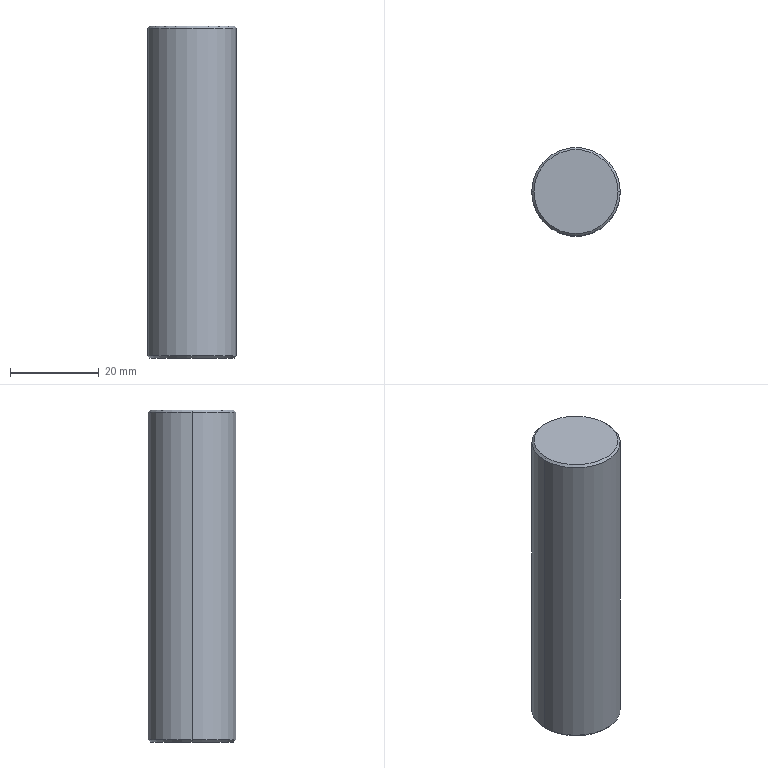Part | Creo | 1 solid | 15 faces | box 20 x 20 x 75 mm | volume 22497 mm3 | cone 6 | cylinder 6 | plane 3 | commonest cylinder face diameters 6.7 x2 8 x2 20 x2
STEP:
#1=CARTESIAN_POINT('',(259.5,184.,-188.491));
#2=VERTEX_POINT('',#1);
#3=CARTESIAN_POINT('',(240.5,184.,-188.491));
#4=VERTEX_POINT('',#3);
#5=CARTESIAN_POINT('',(250.,184.,-188.491));
#6=DIRECTION('',(0.,0.,-1.));
#7=DIRECTION('',(1.,0.,0.));
#8=AXIS2_PLACEMENT_3D('',#5,#6,#7);
#9=CIRCLE('',#8,9.5);
#10=EDGE_CURVE('',#2,#4,#9,.T.);
#11=ORIENTED_EDGE('',*,*,#10,.F.);
#12=CARTESIAN_POINT('',(250.,184.,-188.491));
#13=DIRECTION('',(0.,0.,-1.));
#14=DIRECTION('',(-1.,0.,0.));
#15=AXIS2_PLACEMENT_3D('',#12,#13,#14);
#16=CIRCLE('',#15,9.5);
#17=EDGE_CURVE('',#4,#2,#16,.T.);
#18=ORIENTED_EDGE('',*,*,#17,.F.);
#19=EDGE_LOOP('',(#11,#18));
#20=FACE_OUTER_BOUND('',#19,.F.);
#21=CARTESIAN_POINT('',(246.,184.,-188.491));
#22=VERTEX_POINT('',#21);
#23=CARTESIAN_POINT('',(254.,184.,-188.491));
#24=VERTEX_POINT('',#23);
#25=CARTESIAN_POINT('',(250.,184.,-188.491));
#26=DIRECTION('',(0.,0.,1.));
#27=DIRECTION('',(-1.,0.,0.));
#28=AXIS2_PLACEMENT_3D('',#25,#26,#27);
#29=CIRCLE('',#28,4.);
#30=EDGE_CURVE('',#22,#24,#29,.T.);
#31=ORIENTED_EDGE('',*,*,#30,.F.);
#32=CARTESIAN_POINT('',(250.,184.,-188.491));
#33=DIRECTION('',(0.,0.,1.));
#34=DIRECTION('',(1.,0.,0.));
#35=AXIS2_PLACEMENT_3D('',#32,#33,#34);
#36=CIRCLE('',#35,4.);
#37=EDGE_CURVE('',#24,#22,#36,.T.);
#38=ORIENTED_EDGE('',*,*,#37,.F.);
#39=EDGE_LOOP('',(#31,#38));
#40=FACE_BOUND('',#39,.F.);
#41=CARTESIAN_POINT('',(250.,184.,-188.491));
#42=DIRECTION('',(0.,0.,-1.));
#43=DIRECTION('',(-1.,0.,0.));
#44=AXIS2_PLACEMENT_3D('',#41,#42,#43);
#45=PLANE('',#44);
#46=ADVANCED_FACE('',(#20,#40),#45,.T.);
#47=ORIENTED_EDGE('',*,*,#10,.T.);
#48=CARTESIAN_POINT('',(240.,184.,-187.991));
#49=VERTEX_POINT('',#48);
#50=CARTESIAN_POINT('',(240.5,184.,-188.491));
#51=DIRECTION('',(-0.7071,0.,0.7071));
#52=VECTOR('',#51,0.7071);
#53=LINE('',#50,#52);
#54=EDGE_CURVE('',#4,#49,#53,.T.);
#55=ORIENTED_EDGE('',*,*,#54,.T.);
#56=CARTESIAN_POINT('',(260.,184.,-187.991));
#57=VERTEX_POINT('',#56);
#58=CARTESIAN_POINT('',(250.,184.,-187.991));
#59=DIRECTION('',(0.,0.,-1.));
#60=DIRECTION('',(1.,0.,0.));
#61=AXIS2_PLACEMENT_3D('',#58,#59,#60);
#62=CIRCLE('',#61,10.);
#63=EDGE_CURVE('',#57,#49,#62,.T.);
#64=ORIENTED_EDGE('',*,*,#63,.F.);
#65=CARTESIAN_POINT('',(259.5,184.,-188.491));
#66=DIRECTION('',(0.7071,0.,0.7071));
#67=VECTOR('',#66,0.7071);
#68=LINE('',#65,#67);
#69=EDGE_CURVE('',#2,#57,#68,.T.);
#70=ORIENTED_EDGE('',*,*,#69,.F.);
#71=EDGE_LOOP('',(#47,#55,#64,#70));
#72=FACE_OUTER_BOUND('',#71,.F.);
#73=CARTESIAN_POINT('',(250.,184.,-188.241));
#74=DIRECTION('',(0.,0.,1.));
#75=DIRECTION('',(1.,0.,0.));
#76=AXIS2_PLACEMENT_3D('',#73,#74,#75);
#77=CONICAL_SURFACE('',#76,9.75,45.);
#78=ADVANCED_FACE('',(#72),#77,.T.);
#79=ORIENTED_EDGE('',*,*,#17,.T.);
#80=ORIENTED_EDGE('',*,*,#69,.T.);
#81=CARTESIAN_POINT('',(250.,184.,-187.991));
#82=DIRECTION('',(0.,0.,-1.));
#83=DIRECTION('',(-1.,0.,0.));
#84=AXIS2_PLACEMENT_3D('',#81,#82,#83);
#85=CIRCLE('',#84,10.);
#86=EDGE_CURVE('',#49,#57,#85,.T.);
#87=ORIENTED_EDGE('',*,*,#86,.F.);
#88=ORIENTED_EDGE('',*,*,#54,.F.);
#89=EDGE_LOOP('',(#79,#80,#87,#88));
#90=FACE_OUTER_BOUND('',#89,.F.);
#91=CARTESIAN_POINT('',(250.,184.,-188.241));
#92=DIRECTION('',(0.,0.,1.));
#93=DIRECTION('',(1.,0.,0.));
#94=AXIS2_PLACEMENT_3D('',#91,#92,#93);
#95=CONICAL_SURFACE('',#94,9.75,45.);
#96=ADVANCED_FACE('',(#90),#95,.T.);
#97=CARTESIAN_POINT('',(260.,184.,-113.991));
#98=VERTEX_POINT('',#97);
#99=CARTESIAN_POINT('',(240.,184.,-113.991));
#100=VERTEX_POINT('',#99);
#101=CARTESIAN_POINT('',(250.,184.,-113.991));
#102=DIRECTION('',(0.,0.,1.));
#103=DIRECTION('',(1.,0.,0.));
#104=AXIS2_PLACEMENT_3D('',#101,#102,#103);
#105=CIRCLE('',#104,10.);
#106=EDGE_CURVE('',#98,#100,#105,.T.);
#107=ORIENTED_EDGE('',*,*,#106,.T.);
#108=CARTESIAN_POINT('',(240.,184.,-187.991));
#109=DIRECTION('',(0.,0.,1.));
#110=VECTOR('',#109,74.);
#111=LINE('',#108,#110);
#112=EDGE_CURVE('',#49,#100,#111,.T.);
#113=ORIENTED_EDGE('',*,*,#112,.F.);
#114=ORIENTED_EDGE('',*,*,#86,.T.);
#115=CARTESIAN_POINT('',(260.,184.,-187.991));
#116=DIRECTION('',(0.,0.,1.));
#117=VECTOR('',#116,74.);
#118=LINE('',#115,#117);
#119=EDGE_CURVE('',#57,#98,#118,.T.);
#120=ORIENTED_EDGE('',*,*,#119,.T.);
#121=EDGE_LOOP('',(#107,#113,#114,#120));
#122=FACE_OUTER_BOUND('',#121,.F.);
#123=CARTESIAN_POINT('',(250.,184.,-187.991));
#124=DIRECTION('',(0.,0.,1.));
#125=DIRECTION('',(1.,0.,0.));
#126=AXIS2_PLACEMENT_3D('',#123,#124,#125);
#127=CYLINDRICAL_SURFACE('',#126,10.);
#128=ADVANCED_FACE('',(#122),#127,.T.);
#129=CARTESIAN_POINT('',(259.5,184.,-113.491));
#130=VERTEX_POINT('',#129);
#131=CARTESIAN_POINT('',(240.5,184.,-113.491));
#132=VERTEX_POINT('',#131);
#133=CARTESIAN_POINT('',(250.,184.,-113.491));
#134=DIRECTION('',(0.,0.,1.));
#135=DIRECTION('',(1.,0.,0.));
#136=AXIS2_PLACEMENT_3D('',#133,#134,#135);
#137=CIRCLE('',#136,9.5);
#138=EDGE_CURVE('',#130,#132,#137,.T.);
#139=ORIENTED_EDGE('',*,*,#138,.T.);
#140=CARTESIAN_POINT('',(240.5,184.,-113.491));
#141=DIRECTION('',(-0.7071,0.,-0.7071));
#142=VECTOR('',#141,0.7071);
#143=LINE('',#140,#142);
#144=EDGE_CURVE('',#132,#100,#143,.T.);
#145=ORIENTED_EDGE('',*,*,#144,.T.);
#146=ORIENTED_EDGE('',*,*,#106,.F.);
#147=CARTESIAN_POINT('',(259.5,184.,-113.491));
#148=DIRECTION('',(0.7071,0.,-0.7071));
#149=VECTOR('',#148,0.7071);
#150=LINE('',#147,#149);
#151=EDGE_CURVE('',#130,#98,#150,.T.);
#152=ORIENTED_EDGE('',*,*,#151,.F.);
#153=EDGE_LOOP('',(#139,#145,#146,#152));
#154=FACE_OUTER_BOUND('',#153,.F.);
#155=CARTESIAN_POINT('',(250.,184.,-113.741));
#156=DIRECTION('',(0.,0.,-1.));
#157=DIRECTION('',(-1.,0.,0.));
#158=AXIS2_PLACEMENT_3D('',#155,#156,#157);
#159=CONICAL_SURFACE('',#158,9.75,45.);
#160=ADVANCED_FACE('',(#154),#159,.T.);
#161=CARTESIAN_POINT('',(250.,184.,-113.491));
#162=DIRECTION('',(0.,0.,1.));
#163=DIRECTION('',(-1.,0.,0.));
#164=AXIS2_PLACEMENT_3D('',#161,#162,#163);
#165=CIRCLE('',#164,9.5);
#166=EDGE_CURVE('',#132,#130,#165,.T.);
#167=ORIENTED_EDGE('',*,*,#166,.F.);
#168=ORIENTED_EDGE('',*,*,#138,.F.);
#169=EDGE_LOOP('',(#167,#168));
#170=FACE_OUTER_BOUND('',#169,.F.);
#171=CARTESIAN_POINT('',(250.,184.,-113.491));
#172=DIRECTION('',(0.,0.,1.));
#173=DIRECTION('',(1.,0.,0.));
#174=AXIS2_PLACEMENT_3D('',#171,#172,#173);
#175=PLANE('',#174);
#176=ADVANCED_FACE('',(#170),#175,.T.);
#177=ORIENTED_EDGE('',*,*,#166,.T.);
#178=ORIENTED_EDGE('',*,*,#151,.T.);
#179=CARTESIAN_POINT('',(250.,184.,-113.991));
#180=DIRECTION('',(0.,0.,1.));
#181=DIRECTION('',(-1.,0.,0.));
#182=AXIS2_PLACEMENT_3D('',#179,#180,#181);
#183=CIRCLE('',#182,10.);
#184=EDGE_CURVE('',#100,#98,#183,.T.);
#185=ORIENTED_EDGE('',*,*,#184,.F.);
#186=ORIENTED_EDGE('',*,*,#144,.F.);
#187=EDGE_LOOP('',(#177,#178,#185,#186));
#188=FACE_OUTER_BOUND('',#187,.F.);
#189=CARTESIAN_POINT('',(250.,184.,-113.741));
#190=DIRECTION('',(0.,0.,-1.));
#191=DIRECTION('',(-1.,0.,0.));
#192=AXIS2_PLACEMENT_3D('',#189,#190,#191);
#193=CONICAL_SURFACE('',#192,9.75,45.);
#194=ADVANCED_FACE('',(#188),#193,.T.);
#195=ORIENTED_EDGE('',*,*,#184,.T.);
#196=ORIENTED_EDGE('',*,*,#119,.F.);
#197=ORIENTED_EDGE('',*,*,#63,.T.);
#198=ORIENTED_EDGE('',*,*,#112,.T.);
#199=EDGE_LOOP('',(#195,#196,#197,#198));
#200=FACE_OUTER_BOUND('',#199,.F.);
#201=CARTESIAN_POINT('',(250.,184.,-187.991));
#202=DIRECTION('',(0.,0.,1.));
#203=DIRECTION('',(1.,0.,0.));
#204=AXIS2_PLACEMENT_3D('',#201,#202,#203);
#205=CYLINDRICAL_SURFACE('',#204,10.);
#206=ADVANCED_FACE('',(#200),#205,.T.);
#207=CARTESIAN_POINT('',(254.,184.,-169.491));
#208=VERTEX_POINT('',#207);
#209=CARTESIAN_POINT('',(246.,184.,-169.491));
#210=VERTEX_POINT('',#209);
#211=CARTESIAN_POINT('',(250.,184.,-169.491));
#212=DIRECTION('',(0.,0.,-1.));
#213=DIRECTION('',(1.,0.,0.));
#214=AXIS2_PLACEMENT_3D('',#211,#212,#213);
#215=CIRCLE('',#214,4.);
#216=EDGE_CURVE('',#208,#210,#215,.T.);
#217=ORIENTED_EDGE('',*,*,#216,.T.);
#218=CARTESIAN_POINT('',(246.,184.,-188.491));
#219=DIRECTION('',(0.,0.,1.));
#220=VECTOR('',#219,19.);
#221=LINE('',#218,#220);
#222=EDGE_CURVE('',#22,#210,#221,.T.);
#223=ORIENTED_EDGE('',*,*,#222,.F.);
#224=ORIENTED_EDGE('',*,*,#30,.T.);
#225=CARTESIAN_POINT('',(254.,184.,-188.491));
#226=DIRECTION('',(0.,0.,1.));
#227=VECTOR('',#226,19.);
#228=LINE('',#225,#227);
#229=EDGE_CURVE('',#24,#208,#228,.T.);
#230=ORIENTED_EDGE('',*,*,#229,.T.);
#231=EDGE_LOOP('',(#217,#223,#224,#230));
#232=FACE_OUTER_BOUND('',#231,.F.);
#233=CARTESIAN_POINT('',(250.,184.,-188.491));
#234=DIRECTION('',(0.,0.,1.));
#235=DIRECTION('',(1.,0.,0.));
#236=AXIS2_PLACEMENT_3D('',#233,#234,#235);
#237=CYLINDRICAL_SURFACE('',#236,4.);
#238=ADVANCED_FACE('',(#232),#237,.F.);
#239=CARTESIAN_POINT('',(250.,184.,-169.491));
#240=DIRECTION('',(0.,0.,-1.));
#241=DIRECTION('',(-1.,0.,0.));
#242=AXIS2_PLACEMENT_3D('',#239,#240,#241);
#243=CIRCLE('',#242,4.);
#244=EDGE_CURVE('',#210,#208,#243,.T.);
#245=ORIENTED_EDGE('',*,*,#244,.F.);
#246=ORIENTED_EDGE('',*,*,#216,.F.);
#247=EDGE_LOOP('',(#245,#246));
#248=FACE_OUTER_BOUND('',#247,.F.);
#249=CARTESIAN_POINT('',(253.35,184.,-169.491));
#250=VERTEX_POINT('',#249);
#251=CARTESIAN_POINT('',(246.65,184.,-169.491));
#252=VERTEX_POINT('',#251);
#253=CARTESIAN_POINT('',(250.,184.,-169.491));
#254=DIRECTION('',(0.,0.,1.));
#255=DIRECTION('',(1.,0.,0.));
#256=AXIS2_PLACEMENT_3D('',#253,#254,#255);
#257=CIRCLE('',#256,3.35);
#258=EDGE_CURVE('',#250,#252,#257,.T.);
#259=ORIENTED_EDGE('',*,*,#258,.F.);
#260=CARTESIAN_POINT('',(250.,184.,-169.491));
#261=DIRECTION('',(0.,0.,1.));
#262=DIRECTION('',(-1.,0.,0.));
#263=AXIS2_PLACEMENT_3D('',#260,#261,#262);
#264=CIRCLE('',#263,3.35);
#265=EDGE_CURVE('',#252,#250,#264,.T.);
#266=ORIENTED_EDGE('',*,*,#265,.F.);
#267=EDGE_LOOP('',(#259,#266));
#268=FACE_BOUND('',#267,.F.);
#269=CARTESIAN_POINT('',(250.,184.,-169.491));
#270=DIRECTION('',(0.,0.,1.));
#271=DIRECTION('',(1.,0.,0.));
#272=AXIS2_PLACEMENT_3D('',#269,#270,#271);
#273=PLANE('',#272);
#274=ADVANCED_FACE('',(#248,#268),#273,.F.);
#275=ORIENTED_EDGE('',*,*,#258,.T.);
#276=CARTESIAN_POINT('',(246.65,184.,-167.491));
#277=VERTEX_POINT('',#276);
#278=CARTESIAN_POINT('',(246.65,184.,-169.491));
#279=DIRECTION('',(0.,0.,1.));
#280=VECTOR('',#279,2.);
#281=LINE('',#278,#280);
#282=EDGE_CURVE('',#252,#277,#281,.T.);
#283=ORIENTED_EDGE('',*,*,#282,.T.);
#284=CARTESIAN_POINT('',(253.35,184.,-167.491));
#285=VERTEX_POINT('',#284);
#286=CARTESIAN_POINT('',(250.,184.,-167.491));
#287=DIRECTION('',(0.,0.,-1.));
#288=DIRECTION('',(-1.,0.,0.));
#289=AXIS2_PLACEMENT_3D('',#286,#287,#288);
#290=CIRCLE('',#289,3.35);
#291=EDGE_CURVE('',#277,#285,#290,.T.);
#292=ORIENTED_EDGE('',*,*,#291,.T.);
#293=CARTESIAN_POINT('',(253.35,184.,-169.491));
#294=DIRECTION('',(0.,0.,1.));
#295=VECTOR('',#294,2.);
#296=LINE('',#293,#295);
#297=EDGE_CURVE('',#250,#285,#296,.T.);
#298=ORIENTED_EDGE('',*,*,#297,.F.);
#299=EDGE_LOOP('',(#275,#283,#292,#298));
#300=FACE_OUTER_BOUND('',#299,.F.);
#301=CARTESIAN_POINT('',(250.,184.,-188.491));
#302=DIRECTION('',(0.,0.,1.));
#303=DIRECTION('',(1.,0.,0.));
#304=AXIS2_PLACEMENT_3D('',#301,#302,#303);
#305=CYLINDRICAL_SURFACE('',#304,3.35);
#306=ADVANCED_FACE('',(#300),#305,.F.);
#307=ORIENTED_EDGE('',*,*,#265,.T.);
#308=ORIENTED_EDGE('',*,*,#297,.T.);
#309=CARTESIAN_POINT('',(250.,184.,-167.491));
#310=DIRECTION('',(0.,0.,-1.));
#311=DIRECTION('',(1.,0.,0.));
#312=AXIS2_PLACEMENT_3D('',#309,#310,#311);
#313=CIRCLE('',#312,3.35);
#314=EDGE_CURVE('',#285,#277,#313,.T.);
#315=ORIENTED_EDGE('',*,*,#314,.T.);
#316=ORIENTED_EDGE('',*,*,#282,.F.);
#317=EDGE_LOOP('',(#307,#308,#315,#316));
#318=FACE_OUTER_BOUND('',#317,.F.);
#319=CARTESIAN_POINT('',(250.,184.,-188.491));
#320=DIRECTION('',(0.,0.,1.));
#321=DIRECTION('',(1.,0.,0.));
#322=AXIS2_PLACEMENT_3D('',#319,#320,#321);
#323=CYLINDRICAL_SURFACE('',#322,3.35);
#324=ADVANCED_FACE('',(#318),#323,.F.);
#325=ORIENTED_EDGE('',*,*,#314,.F.);
#326=CARTESIAN_POINT('',(250.,184.,-165.479));
#327=VERTEX_POINT('',#326);
#328=CARTESIAN_POINT('',(250.,184.,-165.479));
#329=DIRECTION('',(0.8572,0.,-0.515));
#330=VECTOR('',#329,3.908);
#331=LINE('',#328,#330);
#332=EDGE_CURVE('',#327,#285,#331,.T.);
#333=ORIENTED_EDGE('',*,*,#332,.F.);
#334=CARTESIAN_POINT('',(250.,184.,-165.479));
#335=DIRECTION('',(-0.8572,0.,-0.515));
#336=VECTOR('',#335,3.908);
#337=LINE('',#334,#336);
#338=EDGE_CURVE('',#327,#277,#337,.T.);
#339=ORIENTED_EDGE('',*,*,#338,.T.);
#340=EDGE_LOOP('',(#325,#333,#339));
#341=FACE_OUTER_BOUND('',#340,.F.);
#342=CARTESIAN_POINT('',(250.,184.,-166.51));
#343=DIRECTION('',(0.,0.,-1.));
#344=DIRECTION('',(-1.,0.,0.));
#345=AXIS2_PLACEMENT_3D('',#342,#343,#344);
#346=CONICAL_SURFACE('',#345,1.716,59.);
#347=ADVANCED_FACE('',(#341),#346,.F.);
#348=ORIENTED_EDGE('',*,*,#291,.F.);
#349=ORIENTED_EDGE('',*,*,#338,.F.);
#350=ORIENTED_EDGE('',*,*,#332,.T.);
#351=EDGE_LOOP('',(#348,#349,#350));
#352=FACE_OUTER_BOUND('',#351,.F.);
#353=CARTESIAN_POINT('',(250.,184.,-166.51));
#354=DIRECTION('',(0.,0.,-1.));
#355=DIRECTION('',(-1.,0.,0.));
#356=AXIS2_PLACEMENT_3D('',#353,#354,#355);
#357=CONICAL_SURFACE('',#356,1.716,59.);
#358=ADVANCED_FACE('',(#352),#357,.F.);
#359=ORIENTED_EDGE('',*,*,#244,.T.);
#360=ORIENTED_EDGE('',*,*,#229,.F.);
#361=ORIENTED_EDGE('',*,*,#37,.T.);
#362=ORIENTED_EDGE('',*,*,#222,.T.);
#363=EDGE_LOOP('',(#359,#360,#361,#362));
#364=FACE_OUTER_BOUND('',#363,.F.);
#365=CARTESIAN_POINT('',(250.,184.,-188.491));
#366=DIRECTION('',(0.,0.,1.));
#367=DIRECTION('',(1.,0.,0.));
#368=AXIS2_PLACEMENT_3D('',#365,#366,#367);
#369=CYLINDRICAL_SURFACE('',#368,4.);
#370=ADVANCED_FACE('',(#364),#369,.F.);
#371=CLOSED_SHELL('',(#46,#78,#96,#128,#160,#176,#194,#206,#238,#274,#306,#324,#347,#358,#370));
#372=MANIFOLD_SOLID_BREP('',#371);
#373=(LENGTH_UNIT()NAMED_UNIT(*)SI_UNIT(.MILLI.,.METRE.));
#374=UNCERTAINTY_MEASURE_WITH_UNIT(LENGTH_MEASURE(0.008015),#373,'','');
#375=(NAMED_UNIT(*)PLANE_ANGLE_UNIT()SI_UNIT($,.RADIAN.));
#376=PLANE_ANGLE_MEASURE_WITH_UNIT(PLANE_ANGLE_MEASURE(0.01745),#375);
#377=(CONVERSION_BASED_UNIT('DEGREE',#376)NAMED_UNIT(*)PLANE_ANGLE_UNIT());
#378=(NAMED_UNIT(*)SI_UNIT($,.STERADIAN.)SOLID_ANGLE_UNIT());
#379=(GEOMETRIC_REPRESENTATION_CONTEXT(3)GLOBAL_UNCERTAINTY_ASSIGNED_CONTEXT((#374))GLOBAL_UNIT_ASSIGNED_CONTEXT((#373,#377,#378))REPRESENTATION_CONTEXT('',''));
#380=ADVANCED_BREP_SHAPE_REPRESENTATION('',(#372),#379);